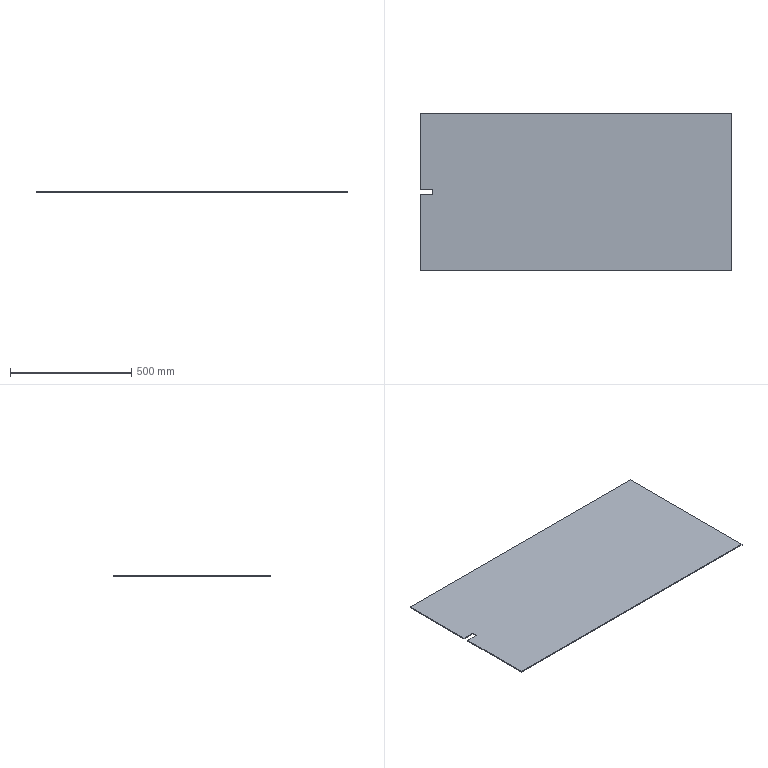Part | SolidWorks | features Extrusion 1 | 1 solid | 10 faces | box 1286 x 652 x 4 mm | volume 3349488 mm3 | plane 10
STEP:
#1=CARTESIAN_POINT('',(0.,315.,0.));
#2=VERTEX_POINT('',#1);
#3=CARTESIAN_POINT('',(0.,0.,0.));
#4=VERTEX_POINT('',#3);
#5=CARTESIAN_POINT('',(0.,0.,0.));
#6=DIRECTION('',(0.,-1.,0.));
#7=VECTOR('',#6,1000.);
#8=LINE('',#5,#7);
#9=EDGE_CURVE('',#2,#4,#8,.T.);
#10=ORIENTED_EDGE('',*,*,#9,.T.);
#11=CARTESIAN_POINT('',(0.,0.,4.));
#12=VERTEX_POINT('',#11);
#13=CARTESIAN_POINT('',(0.,0.,4.));
#14=DIRECTION('',(0.,0.,-1.));
#15=VECTOR('',#14,1000.);
#16=LINE('',#13,#15);
#17=EDGE_CURVE('',#12,#4,#16,.T.);
#18=ORIENTED_EDGE('',*,*,#17,.F.);
#19=CARTESIAN_POINT('',(0.,315.,4.));
#20=VERTEX_POINT('',#19);
#21=CARTESIAN_POINT('',(0.,0.,4.));
#22=DIRECTION('',(0.,-1.,0.));
#23=VECTOR('',#22,1000.);
#24=LINE('',#21,#23);
#25=EDGE_CURVE('',#20,#12,#24,.T.);
#26=ORIENTED_EDGE('',*,*,#25,.F.);
#27=CARTESIAN_POINT('',(0.,315.,4.));
#28=DIRECTION('',(0.,0.,-1.));
#29=VECTOR('',#28,1000.);
#30=LINE('',#27,#29);
#31=EDGE_CURVE('',#20,#2,#30,.T.);
#32=ORIENTED_EDGE('',*,*,#31,.T.);
#33=EDGE_LOOP('',(#10,#18,#26,#32));
#34=FACE_OUTER_BOUND('',#33,.T.);
#35=CARTESIAN_POINT('',(0.,0.,4.));
#36=DIRECTION('',(1.,0.,0.));
#37=DIRECTION('',(0.,0.,-1.));
#38=AXIS2_PLACEMENT_3D('',#35,#36,#37);
#39=PLANE('',#38);
#40=ADVANCED_FACE('',(#34),#39,.F.);
#41=CARTESIAN_POINT('',(1286.,0.,0.));
#42=VERTEX_POINT('',#41);
#43=CARTESIAN_POINT('',(0.,0.,0.));
#44=DIRECTION('',(1.,0.,0.));
#45=VECTOR('',#44,1000.);
#46=LINE('',#43,#45);
#47=EDGE_CURVE('',#4,#42,#46,.T.);
#48=ORIENTED_EDGE('',*,*,#47,.T.);
#49=CARTESIAN_POINT('',(1286.,0.,4.));
#50=VERTEX_POINT('',#49);
#51=CARTESIAN_POINT('',(1286.,0.,4.));
#52=DIRECTION('',(0.,0.,-1.));
#53=VECTOR('',#52,1000.);
#54=LINE('',#51,#53);
#55=EDGE_CURVE('',#50,#42,#54,.T.);
#56=ORIENTED_EDGE('',*,*,#55,.F.);
#57=CARTESIAN_POINT('',(0.,0.,4.));
#58=DIRECTION('',(1.,0.,0.));
#59=VECTOR('',#58,1000.);
#60=LINE('',#57,#59);
#61=EDGE_CURVE('',#12,#50,#60,.T.);
#62=ORIENTED_EDGE('',*,*,#61,.F.);
#63=ORIENTED_EDGE('',*,*,#17,.T.);
#64=EDGE_LOOP('',(#48,#56,#62,#63));
#65=FACE_OUTER_BOUND('',#64,.T.);
#66=CARTESIAN_POINT('',(0.,0.,4.));
#67=DIRECTION('',(0.,1.,0.));
#68=DIRECTION('',(0.,0.,1.));
#69=AXIS2_PLACEMENT_3D('',#66,#67,#68);
#70=PLANE('',#69);
#71=ADVANCED_FACE('',(#65),#70,.F.);
#72=CARTESIAN_POINT('',(1286.,652.,0.));
#73=VERTEX_POINT('',#72);
#74=CARTESIAN_POINT('',(1286.,0.,0.));
#75=DIRECTION('',(0.,1.,0.));
#76=VECTOR('',#75,1000.);
#77=LINE('',#74,#76);
#78=EDGE_CURVE('',#42,#73,#77,.T.);
#79=ORIENTED_EDGE('',*,*,#78,.T.);
#80=CARTESIAN_POINT('',(1286.,652.,4.));
#81=VERTEX_POINT('',#80);
#82=CARTESIAN_POINT('',(1286.,652.,4.));
#83=DIRECTION('',(0.,0.,-1.));
#84=VECTOR('',#83,1000.);
#85=LINE('',#82,#84);
#86=EDGE_CURVE('',#81,#73,#85,.T.);
#87=ORIENTED_EDGE('',*,*,#86,.F.);
#88=CARTESIAN_POINT('',(1286.,0.,4.));
#89=DIRECTION('',(0.,1.,0.));
#90=VECTOR('',#89,1000.);
#91=LINE('',#88,#90);
#92=EDGE_CURVE('',#50,#81,#91,.T.);
#93=ORIENTED_EDGE('',*,*,#92,.F.);
#94=ORIENTED_EDGE('',*,*,#55,.T.);
#95=EDGE_LOOP('',(#79,#87,#93,#94));
#96=FACE_OUTER_BOUND('',#95,.T.);
#97=CARTESIAN_POINT('',(1286.,0.,4.));
#98=DIRECTION('',(-1.,0.,0.));
#99=DIRECTION('',(0.,0.,1.));
#100=AXIS2_PLACEMENT_3D('',#97,#98,#99);
#101=PLANE('',#100);
#102=ADVANCED_FACE('',(#96),#101,.F.);
#103=CARTESIAN_POINT('',(0.,652.,0.));
#104=VERTEX_POINT('',#103);
#105=CARTESIAN_POINT('',(0.,652.,0.));
#106=DIRECTION('',(-1.,0.,0.));
#107=VECTOR('',#106,1000.);
#108=LINE('',#105,#107);
#109=EDGE_CURVE('',#73,#104,#108,.T.);
#110=ORIENTED_EDGE('',*,*,#109,.T.);
#111=CARTESIAN_POINT('',(0.,652.,4.));
#112=VERTEX_POINT('',#111);
#113=CARTESIAN_POINT('',(0.,652.,4.));
#114=DIRECTION('',(0.,0.,-1.));
#115=VECTOR('',#114,1000.);
#116=LINE('',#113,#115);
#117=EDGE_CURVE('',#112,#104,#116,.T.);
#118=ORIENTED_EDGE('',*,*,#117,.F.);
#119=CARTESIAN_POINT('',(0.,652.,4.));
#120=DIRECTION('',(-1.,0.,0.));
#121=VECTOR('',#120,1000.);
#122=LINE('',#119,#121);
#123=EDGE_CURVE('',#81,#112,#122,.T.);
#124=ORIENTED_EDGE('',*,*,#123,.F.);
#125=ORIENTED_EDGE('',*,*,#86,.T.);
#126=EDGE_LOOP('',(#110,#118,#124,#125));
#127=FACE_OUTER_BOUND('',#126,.T.);
#128=CARTESIAN_POINT('',(0.,652.,4.));
#129=DIRECTION('',(0.,-1.,0.));
#130=DIRECTION('',(0.,0.,-1.));
#131=AXIS2_PLACEMENT_3D('',#128,#129,#130);
#132=PLANE('',#131);
#133=ADVANCED_FACE('',(#127),#132,.F.);
#134=CARTESIAN_POINT('',(0.,337.,0.));
#135=VERTEX_POINT('',#134);
#136=CARTESIAN_POINT('',(0.,337.,0.));
#137=DIRECTION('',(0.,-1.,0.));
#138=VECTOR('',#137,1000.);
#139=LINE('',#136,#138);
#140=EDGE_CURVE('',#104,#135,#139,.T.);
#141=ORIENTED_EDGE('',*,*,#140,.T.);
#142=CARTESIAN_POINT('',(0.,337.,4.));
#143=VERTEX_POINT('',#142);
#144=CARTESIAN_POINT('',(0.,337.,4.));
#145=DIRECTION('',(0.,0.,-1.));
#146=VECTOR('',#145,1000.);
#147=LINE('',#144,#146);
#148=EDGE_CURVE('',#143,#135,#147,.T.);
#149=ORIENTED_EDGE('',*,*,#148,.F.);
#150=CARTESIAN_POINT('',(0.,337.,4.));
#151=DIRECTION('',(0.,-1.,0.));
#152=VECTOR('',#151,1000.);
#153=LINE('',#150,#152);
#154=EDGE_CURVE('',#112,#143,#153,.T.);
#155=ORIENTED_EDGE('',*,*,#154,.F.);
#156=ORIENTED_EDGE('',*,*,#117,.T.);
#157=EDGE_LOOP('',(#141,#149,#155,#156));
#158=FACE_OUTER_BOUND('',#157,.T.);
#159=CARTESIAN_POINT('',(0.,337.,4.));
#160=DIRECTION('',(1.,0.,0.));
#161=DIRECTION('',(0.,0.,-1.));
#162=AXIS2_PLACEMENT_3D('',#159,#160,#161);
#163=PLANE('',#162);
#164=ADVANCED_FACE('',(#158),#163,.F.);
#165=CARTESIAN_POINT('',(50.,337.,0.));
#166=VERTEX_POINT('',#165);
#167=CARTESIAN_POINT('',(50.,337.,0.));
#168=DIRECTION('',(1.,0.,0.));
#169=VECTOR('',#168,1000.);
#170=LINE('',#167,#169);
#171=EDGE_CURVE('',#135,#166,#170,.T.);
#172=ORIENTED_EDGE('',*,*,#171,.T.);
#173=CARTESIAN_POINT('',(50.,337.,4.));
#174=VERTEX_POINT('',#173);
#175=CARTESIAN_POINT('',(50.,337.,4.));
#176=DIRECTION('',(0.,0.,-1.));
#177=VECTOR('',#176,1000.);
#178=LINE('',#175,#177);
#179=EDGE_CURVE('',#174,#166,#178,.T.);
#180=ORIENTED_EDGE('',*,*,#179,.F.);
#181=CARTESIAN_POINT('',(50.,337.,4.));
#182=DIRECTION('',(1.,0.,0.));
#183=VECTOR('',#182,1000.);
#184=LINE('',#181,#183);
#185=EDGE_CURVE('',#143,#174,#184,.T.);
#186=ORIENTED_EDGE('',*,*,#185,.F.);
#187=ORIENTED_EDGE('',*,*,#148,.T.);
#188=EDGE_LOOP('',(#172,#180,#186,#187));
#189=FACE_OUTER_BOUND('',#188,.T.);
#190=CARTESIAN_POINT('',(50.,337.,4.));
#191=DIRECTION('',(0.,1.,0.));
#192=DIRECTION('',(0.,0.,1.));
#193=AXIS2_PLACEMENT_3D('',#190,#191,#192);
#194=PLANE('',#193);
#195=ADVANCED_FACE('',(#189),#194,.F.);
#196=CARTESIAN_POINT('',(50.,315.,0.));
#197=VERTEX_POINT('',#196);
#198=CARTESIAN_POINT('',(50.,315.,0.));
#199=DIRECTION('',(0.,-1.,0.));
#200=VECTOR('',#199,1000.);
#201=LINE('',#198,#200);
#202=EDGE_CURVE('',#166,#197,#201,.T.);
#203=ORIENTED_EDGE('',*,*,#202,.T.);
#204=CARTESIAN_POINT('',(50.,315.,4.));
#205=VERTEX_POINT('',#204);
#206=CARTESIAN_POINT('',(50.,315.,4.));
#207=DIRECTION('',(0.,0.,-1.));
#208=VECTOR('',#207,1000.);
#209=LINE('',#206,#208);
#210=EDGE_CURVE('',#205,#197,#209,.T.);
#211=ORIENTED_EDGE('',*,*,#210,.F.);
#212=CARTESIAN_POINT('',(50.,315.,4.));
#213=DIRECTION('',(0.,-1.,0.));
#214=VECTOR('',#213,1000.);
#215=LINE('',#212,#214);
#216=EDGE_CURVE('',#174,#205,#215,.T.);
#217=ORIENTED_EDGE('',*,*,#216,.F.);
#218=ORIENTED_EDGE('',*,*,#179,.T.);
#219=EDGE_LOOP('',(#203,#211,#217,#218));
#220=FACE_OUTER_BOUND('',#219,.T.);
#221=CARTESIAN_POINT('',(50.,315.,4.));
#222=DIRECTION('',(1.,0.,0.));
#223=DIRECTION('',(0.,0.,-1.));
#224=AXIS2_PLACEMENT_3D('',#221,#222,#223);
#225=PLANE('',#224);
#226=ADVANCED_FACE('',(#220),#225,.F.);
#227=CARTESIAN_POINT('',(0.,315.,0.));
#228=DIRECTION('',(-1.,0.,0.));
#229=VECTOR('',#228,1000.);
#230=LINE('',#227,#229);
#231=EDGE_CURVE('',#197,#2,#230,.T.);
#232=ORIENTED_EDGE('',*,*,#231,.T.);
#233=ORIENTED_EDGE('',*,*,#31,.F.);
#234=CARTESIAN_POINT('',(0.,315.,4.));
#235=DIRECTION('',(-1.,0.,0.));
#236=VECTOR('',#235,1000.);
#237=LINE('',#234,#236);
#238=EDGE_CURVE('',#205,#20,#237,.T.);
#239=ORIENTED_EDGE('',*,*,#238,.F.);
#240=ORIENTED_EDGE('',*,*,#210,.T.);
#241=EDGE_LOOP('',(#232,#233,#239,#240));
#242=FACE_OUTER_BOUND('',#241,.T.);
#243=CARTESIAN_POINT('',(0.,315.,4.));
#244=DIRECTION('',(0.,-1.,0.));
#245=DIRECTION('',(0.,0.,-1.));
#246=AXIS2_PLACEMENT_3D('',#243,#244,#245);
#247=PLANE('',#246);
#248=ADVANCED_FACE('',(#242),#247,.F.);
#249=ORIENTED_EDGE('',*,*,#25,.T.);
#250=ORIENTED_EDGE('',*,*,#61,.T.);
#251=ORIENTED_EDGE('',*,*,#92,.T.);
#252=ORIENTED_EDGE('',*,*,#123,.T.);
#253=ORIENTED_EDGE('',*,*,#154,.T.);
#254=ORIENTED_EDGE('',*,*,#185,.T.);
#255=ORIENTED_EDGE('',*,*,#216,.T.);
#256=ORIENTED_EDGE('',*,*,#238,.T.);
#257=EDGE_LOOP('',(#249,#250,#251,#252,#253,#254,#255,#256));
#258=FACE_OUTER_BOUND('',#257,.T.);
#259=CARTESIAN_POINT('',(0.,0.,4.));
#260=DIRECTION('',(0.,0.,-1.));
#261=DIRECTION('',(-1.,0.,0.));
#262=AXIS2_PLACEMENT_3D('',#259,#260,#261);
#263=PLANE('',#262);
#264=ADVANCED_FACE('',(#258),#263,.F.);
#265=ORIENTED_EDGE('',*,*,#9,.F.);
#266=ORIENTED_EDGE('',*,*,#231,.F.);
#267=ORIENTED_EDGE('',*,*,#202,.F.);
#268=ORIENTED_EDGE('',*,*,#171,.F.);
#269=ORIENTED_EDGE('',*,*,#140,.F.);
#270=ORIENTED_EDGE('',*,*,#109,.F.);
#271=ORIENTED_EDGE('',*,*,#78,.F.);
#272=ORIENTED_EDGE('',*,*,#47,.F.);
#273=EDGE_LOOP('',(#265,#266,#267,#268,#269,#270,#271,#272));
#274=FACE_OUTER_BOUND('',#273,.T.);
#275=CARTESIAN_POINT('',(0.,0.,0.));
#276=DIRECTION('',(0.,0.,-1.));
#277=DIRECTION('',(-1.,0.,0.));
#278=AXIS2_PLACEMENT_3D('',#275,#276,#277);
#279=PLANE('',#278);
#280=ADVANCED_FACE('',(#274),#279,.T.);
#281=CLOSED_SHELL('',(#40,#71,#102,#133,#164,#195,#226,#248,#264,#280));
#282=MANIFOLD_SOLID_BREP('',#281);
#283=CARTESIAN_POINT('',(0.,0.,0.));
#284=DIRECTION('',(0.,0.,1.));
#285=DIRECTION('',(1.,0.,0.));
#286=AXIS2_PLACEMENT_3D('',#283,#284,#285);
#287=(LENGTH_UNIT()NAMED_UNIT(*)SI_UNIT(.MILLI.,.METRE.));
#288=UNCERTAINTY_MEASURE_WITH_UNIT(LENGTH_MEASURE(0.00001),#287,'','');
#289=(NAMED_UNIT(*)PLANE_ANGLE_UNIT()SI_UNIT($,.RADIAN.));
#290=(NAMED_UNIT(*)SI_UNIT($,.STERADIAN.)SOLID_ANGLE_UNIT());
#291=(GEOMETRIC_REPRESENTATION_CONTEXT(3)GLOBAL_UNCERTAINTY_ASSIGNED_CONTEXT((#288))GLOBAL_UNIT_ASSIGNED_CONTEXT((#287,#289,#290))REPRESENTATION_CONTEXT('',''));
#292=ADVANCED_BREP_SHAPE_REPRESENTATION('',(#282,#286),#291);